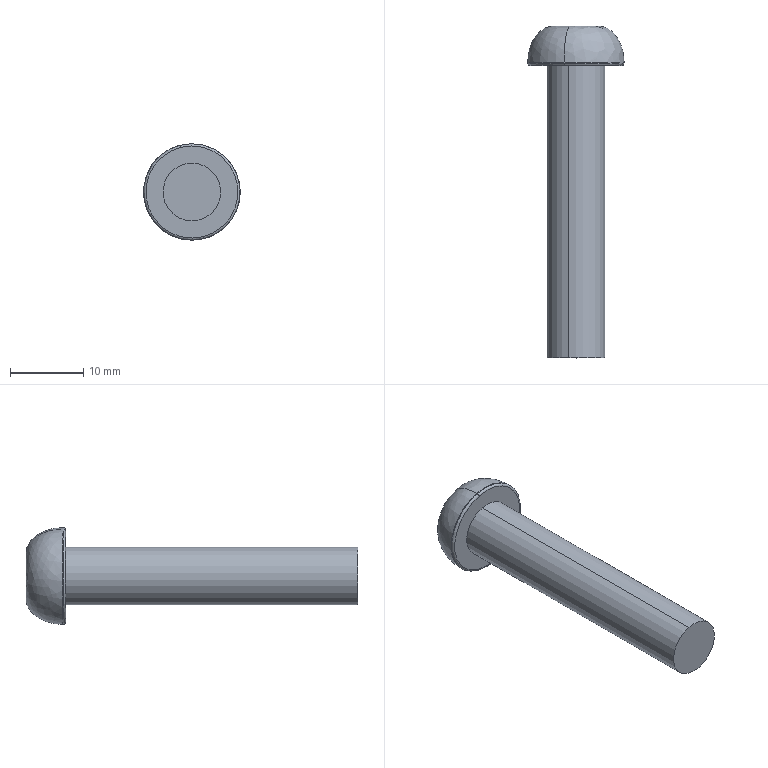Part | SolidWorks | features BaseBody 1 | 1 solid | 23 faces | box 13.2 x 45.4 x 13.2 mm | volume 2505 mm3 | plane 15 | cylinder 4 | torus 2 | spline 2 | commonest cylinder face diameters 7.9 x2 13.2 x2
STEP:
#1=CARTESIAN_POINT('',(-484.292,-107.35,172.017));
#2=VERTEX_POINT('',#1);
#3=CARTESIAN_POINT('',(-486.243,-107.35,179.672));
#4=VERTEX_POINT('',#3);
#5=CARTESIAN_POINT('',(-485.268,-107.35,175.844));
#6=DIRECTION('',(0.,-1.,0.));
#7=DIRECTION('',(0.,0.,-1.));
#8=AXIS2_PLACEMENT_3D('',#5,#6,#7);
#9=CIRCLE('',#8,3.95);
#10=EDGE_CURVE('',#2,#4,#9,.T.);
#11=ORIENTED_EDGE('',*,*,#10,.F.);
#12=CARTESIAN_POINT('',(-484.292,-67.35,172.017));
#13=VERTEX_POINT('',#12);
#14=CARTESIAN_POINT('',(-484.292,-79.35,172.017));
#15=DIRECTION('',(0.,1.,0.));
#16=VECTOR('',#15,1000.);
#17=LINE('',#14,#16);
#18=EDGE_CURVE('',#2,#13,#17,.T.);
#19=ORIENTED_EDGE('',*,*,#18,.T.);
#20=CARTESIAN_POINT('',(-486.243,-67.35,179.672));
#21=VERTEX_POINT('',#20);
#22=CARTESIAN_POINT('',(-485.268,-67.35,175.844));
#23=DIRECTION('',(0.,1.,0.));
#24=DIRECTION('',(0.,0.,-1.));
#25=AXIS2_PLACEMENT_3D('',#22,#23,#24);
#26=CIRCLE('',#25,3.95);
#27=EDGE_CURVE('',#21,#13,#26,.T.);
#28=ORIENTED_EDGE('',*,*,#27,.F.);
#29=CARTESIAN_POINT('',(-486.243,-79.35,179.672));
#30=DIRECTION('',(0.,1.,0.));
#31=VECTOR('',#30,1000.);
#32=LINE('',#29,#31);
#33=EDGE_CURVE('',#4,#21,#32,.T.);
#34=ORIENTED_EDGE('',*,*,#33,.F.);
#35=EDGE_LOOP('',(#11,#19,#28,#34));
#36=FACE_OUTER_BOUND('',#35,.T.);
#37=CARTESIAN_POINT('',(-485.268,-79.35,175.844));
#38=DIRECTION('',(0.,1.,0.));
#39=DIRECTION('',(-0.247,0.,0.969));
#40=AXIS2_PLACEMENT_3D('',#37,#38,#39);
#41=CYLINDRICAL_SURFACE('',#40,3.95);
#42=ADVANCED_FACE('',(#36),#41,.T.);
#43=CARTESIAN_POINT('',(-483.638,-67.05,169.449));
#44=VERTEX_POINT('',#43);
#45=CARTESIAN_POINT('',(-486.898,-67.05,182.24));
#46=VERTEX_POINT('',#45);
#47=CARTESIAN_POINT('',(-485.268,-67.05,175.844));
#48=DIRECTION('',(0.,-1.,0.));
#49=DIRECTION('',(0.247,0.,-0.969));
#50=AXIS2_PLACEMENT_3D('',#47,#48,#49);
#51=CIRCLE('',#50,6.6);
#52=EDGE_CURVE('',#44,#46,#51,.T.);
#53=ORIENTED_EDGE('',*,*,#52,.T.);
#54=CARTESIAN_POINT('',(-486.824,-67.35,181.949));
#55=VERTEX_POINT('',#54);
#56=CARTESIAN_POINT('',(-486.824,-67.05,181.949));
#57=DIRECTION('',(0.969,0.,0.247));
#58=DIRECTION('',(0.247,0.,-0.969));
#59=AXIS2_PLACEMENT_3D('',#56,#57,#58);
#60=CIRCLE('',#59,0.3);
#61=EDGE_CURVE('',#46,#55,#60,.T.);
#62=ORIENTED_EDGE('',*,*,#61,.T.);
#63=CARTESIAN_POINT('',(-483.712,-67.35,169.739));
#64=VERTEX_POINT('',#63);
#65=CARTESIAN_POINT('',(-485.268,-67.35,175.844));
#66=DIRECTION('',(0.,-1.,0.));
#67=DIRECTION('',(0.247,0.,-0.969));
#68=AXIS2_PLACEMENT_3D('',#65,#66,#67);
#69=CIRCLE('',#68,6.3);
#70=EDGE_CURVE('',#64,#55,#69,.T.);
#71=ORIENTED_EDGE('',*,*,#70,.F.);
#72=CARTESIAN_POINT('',(-483.712,-67.05,169.739));
#73=DIRECTION('',(-0.969,0.,-0.247));
#74=DIRECTION('',(-0.247,0.,0.969));
#75=AXIS2_PLACEMENT_3D('',#72,#73,#74);
#76=CIRCLE('',#75,0.3);
#77=EDGE_CURVE('',#44,#64,#76,.T.);
#78=ORIENTED_EDGE('',*,*,#77,.F.);
#79=EDGE_LOOP('',(#53,#62,#71,#78));
#80=FACE_OUTER_BOUND('',#79,.T.);
#81=CARTESIAN_POINT('',(-485.268,-67.05,175.844));
#82=DIRECTION('',(0.,-1.,0.));
#83=DIRECTION('',(0.247,0.,-0.969));
#84=AXIS2_PLACEMENT_3D('',#81,#82,#83);
#85=TOROIDAL_SURFACE('',#84,6.3,0.3);
#86=ADVANCED_FACE('',(#80),#85,.T.);
#87=ORIENTED_EDGE('',*,*,#52,.F.);
#88=CARTESIAN_POINT('',(-483.638,-66.95,169.449));
#89=VERTEX_POINT('',#88);
#90=CARTESIAN_POINT('',(-483.638,-67.35,169.449));
#91=DIRECTION('',(0.,1.,0.));
#92=VECTOR('',#91,1000.);
#93=LINE('',#90,#92);
#94=EDGE_CURVE('',#44,#89,#93,.T.);
#95=ORIENTED_EDGE('',*,*,#94,.T.);
#96=CARTESIAN_POINT('',(-486.898,-66.95,182.24));
#97=VERTEX_POINT('',#96);
#98=CARTESIAN_POINT('',(-486.898,-66.95,182.24));
#99=CARTESIAN_POINT('',(-474.107,-66.95,185.5));
#100=CARTESIAN_POINT('',(-470.847,-66.95,172.709));
#101=CARTESIAN_POINT('',(-483.638,-66.95,169.449));
#102=(BOUNDED_CURVE()B_SPLINE_CURVE(3,(#98,#99,#100,#101),.UNSPECIFIED.,.F.,.F.)B_SPLINE_CURVE_WITH_KNOTS((4,4),(0.,1.),.UNSPECIFIED.)CURVE()GEOMETRIC_REPRESENTATION_ITEM()RATIONAL_B_SPLINE_CURVE((1.,0.3333,0.3333,1.))REPRESENTATION_ITEM(''));
#103=EDGE_CURVE('',#97,#89,#102,.T.);
#104=ORIENTED_EDGE('',*,*,#103,.F.);
#105=CARTESIAN_POINT('',(-486.898,-67.35,182.24));
#106=DIRECTION('',(0.,1.,0.));
#107=VECTOR('',#106,1000.);
#108=LINE('',#105,#107);
#109=EDGE_CURVE('',#46,#97,#108,.T.);
#110=ORIENTED_EDGE('',*,*,#109,.F.);
#111=EDGE_LOOP('',(#87,#95,#104,#110));
#112=FACE_OUTER_BOUND('',#111,.T.);
#113=CARTESIAN_POINT('',(-485.268,-67.35,175.844));
#114=DIRECTION('',(0.,1.,0.));
#115=DIRECTION('',(-0.247,0.,0.969));
#116=AXIS2_PLACEMENT_3D('',#113,#114,#115);
#117=CYLINDRICAL_SURFACE('',#116,6.6);
#118=ADVANCED_FACE('',(#112),#117,.T.);
#119=CARTESIAN_POINT('',(-487.296,-64.03,177.923));
#120=VERTEX_POINT('',#119);
#121=CARTESIAN_POINT('',(-485.268,-65.482,175.844));
#122=VERTEX_POINT('',#121);
#123=CARTESIAN_POINT('',(-487.296,-64.03,177.923));
#124=DIRECTION('',(0.6247,-0.4472,-0.6401));
#125=VECTOR('',#124,1000.);
#126=LINE('',#123,#125);
#127=EDGE_CURVE('',#120,#122,#126,.T.);
#128=ORIENTED_EDGE('',*,*,#127,.T.);
#129=CARTESIAN_POINT('',(-488.082,-64.03,175.127));
#130=VERTEX_POINT('',#129);
#131=CARTESIAN_POINT('',(-488.082,-64.03,175.127));
#132=DIRECTION('',(0.8667,-0.4472,0.2209));
#133=VECTOR('',#132,1000.);
#134=LINE('',#131,#133);
#135=EDGE_CURVE('',#130,#122,#134,.T.);
#136=ORIENTED_EDGE('',*,*,#135,.F.);
#137=CARTESIAN_POINT('',(-488.082,-64.03,175.127));
#138=DIRECTION('',(0.2706,0.,0.9627));
#139=VECTOR('',#138,1000.);
#140=LINE('',#137,#139);
#141=EDGE_CURVE('',#130,#120,#140,.T.);
#142=ORIENTED_EDGE('',*,*,#141,.T.);
#143=EDGE_LOOP('',(#128,#136,#142));
#144=FACE_OUTER_BOUND('',#143,.T.);
#145=CARTESIAN_POINT('',(-488.082,-64.03,175.127));
#146=DIRECTION('',(-0.4813,-0.866,0.1353));
#147=DIRECTION('',(-0.8741,0.4858,0.));
#148=AXIS2_PLACEMENT_3D('',#145,#146,#147);
#149=PLANE('',#148);
#150=ADVANCED_FACE('',(#144),#149,.F.);
#151=CARTESIAN_POINT('',(-487.296,-61.95,177.923));
#152=VERTEX_POINT('',#151);
#153=CARTESIAN_POINT('',(-487.296,-61.95,177.923));
#154=DIRECTION('',(0.,-1.,0.));
#155=VECTOR('',#154,1000.);
#156=LINE('',#153,#155);
#157=EDGE_CURVE('',#152,#120,#156,.T.);
#158=ORIENTED_EDGE('',*,*,#157,.T.);
#159=ORIENTED_EDGE('',*,*,#141,.F.);
#160=CARTESIAN_POINT('',(-488.082,-61.95,175.127));
#161=VERTEX_POINT('',#160);
#162=CARTESIAN_POINT('',(-488.082,-61.95,175.127));
#163=DIRECTION('',(0.,-1.,0.));
#164=VECTOR('',#163,1000.);
#165=LINE('',#162,#164);
#166=EDGE_CURVE('',#161,#130,#165,.T.);
#167=ORIENTED_EDGE('',*,*,#166,.F.);
#168=CARTESIAN_POINT('',(-487.296,-61.95,177.923));
#169=DIRECTION('',(-0.2706,0.,-0.9627));
#170=VECTOR('',#169,1000.);
#171=LINE('',#168,#170);
#172=EDGE_CURVE('',#152,#161,#171,.T.);
#173=ORIENTED_EDGE('',*,*,#172,.F.);
#174=EDGE_LOOP('',(#158,#159,#167,#173));
#175=FACE_OUTER_BOUND('',#174,.T.);
#176=CARTESIAN_POINT('',(-488.082,-64.03,175.127));
#177=DIRECTION('',(-0.9627,0.,0.2706));
#178=DIRECTION('',(0.,1.,0.));
#179=AXIS2_PLACEMENT_3D('',#176,#177,#178);
#180=PLANE('',#179);
#181=ADVANCED_FACE('',(#175),#180,.F.);
#182=CARTESIAN_POINT('',(-482.454,-61.95,176.562));
#183=VERTEX_POINT('',#182);
#184=CARTESIAN_POINT('',(-484.482,-61.95,178.64));
#185=VERTEX_POINT('',#184);
#186=CARTESIAN_POINT('',(-482.454,-61.95,176.562));
#187=DIRECTION('',(-0.6984,0.,0.7157));
#188=VECTOR('',#187,1000.);
#189=LINE('',#186,#188);
#190=EDGE_CURVE('',#183,#185,#189,.T.);
#191=ORIENTED_EDGE('',*,*,#190,.T.);
#192=CARTESIAN_POINT('',(-484.482,-61.95,178.64));
#193=DIRECTION('',(-0.969,0.,-0.247));
#194=VECTOR('',#193,1000.);
#195=LINE('',#192,#194);
#196=EDGE_CURVE('',#185,#152,#195,.T.);
#197=ORIENTED_EDGE('',*,*,#196,.T.);
#198=ORIENTED_EDGE('',*,*,#172,.T.);
#199=CARTESIAN_POINT('',(-486.054,-61.95,173.049));
#200=VERTEX_POINT('',#199);
#201=CARTESIAN_POINT('',(-488.082,-61.95,175.127));
#202=DIRECTION('',(0.6984,0.,-0.7157));
#203=VECTOR('',#202,1000.);
#204=LINE('',#201,#203);
#205=EDGE_CURVE('',#161,#200,#204,.T.);
#206=ORIENTED_EDGE('',*,*,#205,.T.);
#207=CARTESIAN_POINT('',(-483.239,-61.95,173.766));
#208=VERTEX_POINT('',#207);
#209=CARTESIAN_POINT('',(-486.054,-61.95,173.049));
#210=DIRECTION('',(0.969,0.,0.247));
#211=VECTOR('',#210,1000.);
#212=LINE('',#209,#211);
#213=EDGE_CURVE('',#200,#208,#212,.T.);
#214=ORIENTED_EDGE('',*,*,#213,.T.);
#215=CARTESIAN_POINT('',(-483.239,-61.95,173.766));
#216=DIRECTION('',(0.2706,0.,0.9627));
#217=VECTOR('',#216,1000.);
#218=LINE('',#215,#217);
#219=EDGE_CURVE('',#208,#183,#218,.T.);
#220=ORIENTED_EDGE('',*,*,#219,.T.);
#221=EDGE_LOOP('',(#191,#197,#198,#206,#214,#220));
#222=FACE_BOUND('',#221,.T.);
#223=CARTESIAN_POINT('',(-484.502,-61.95,172.84));
#224=VERTEX_POINT('',#223);
#225=CARTESIAN_POINT('',(-486.033,-61.95,178.848));
#226=VERTEX_POINT('',#225);
#227=CARTESIAN_POINT('',(-484.502,-61.95,172.84));
#228=CARTESIAN_POINT('',(-484.6,-61.95,172.815));
#229=CARTESIAN_POINT('',(-484.699,-61.95,172.795));
#230=CARTESIAN_POINT('',(-484.899,-61.95,172.765));
#231=CARTESIAN_POINT('',(-485.002,-61.95,172.755));
#232=CARTESIAN_POINT('',(-485.305,-61.95,172.74));
#233=CARTESIAN_POINT('',(-485.509,-61.95,172.75));
#234=CARTESIAN_POINT('',(-485.911,-61.95,172.808));
#235=CARTESIAN_POINT('',(-486.107,-61.95,172.855));
#236=CARTESIAN_POINT('',(-486.492,-61.95,172.99));
#237=CARTESIAN_POINT('',(-486.677,-61.95,173.076));
#238=CARTESIAN_POINT('',(-486.937,-61.95,173.23));
#239=CARTESIAN_POINT('',(-487.021,-61.95,173.286));
#240=CARTESIAN_POINT('',(-487.184,-61.95,173.406));
#241=CARTESIAN_POINT('',(-487.264,-61.95,173.472));
#242=CARTESIAN_POINT('',(-487.489,-61.95,173.675));
#243=CARTESIAN_POINT('',(-487.626,-61.95,173.826));
#244=CARTESIAN_POINT('',(-487.87,-61.95,174.152));
#245=CARTESIAN_POINT('',(-487.974,-61.95,174.324));
#246=CARTESIAN_POINT('',(-488.152,-61.95,174.692));
#247=CARTESIAN_POINT('',(-488.222,-61.95,174.884));
#248=CARTESIAN_POINT('',(-488.297,-61.95,175.176));
#249=CARTESIAN_POINT('',(-488.317,-61.95,175.275));
#250=CARTESIAN_POINT('',(-488.347,-61.95,175.475));
#251=CARTESIAN_POINT('',(-488.357,-61.95,175.579));
#252=CARTESIAN_POINT('',(-488.372,-61.95,175.881));
#253=CARTESIAN_POINT('',(-488.362,-61.95,176.085));
#254=CARTESIAN_POINT('',(-488.304,-61.95,176.487));
#255=CARTESIAN_POINT('',(-488.257,-61.95,176.683));
#256=CARTESIAN_POINT('',(-488.122,-61.95,177.069));
#257=CARTESIAN_POINT('',(-488.036,-61.95,177.254));
#258=CARTESIAN_POINT('',(-487.882,-61.95,177.514));
#259=CARTESIAN_POINT('',(-487.826,-61.95,177.598));
#260=CARTESIAN_POINT('',(-487.706,-61.95,177.76));
#261=CARTESIAN_POINT('',(-487.64,-61.95,177.841));
#262=CARTESIAN_POINT('',(-487.437,-61.95,178.065));
#263=CARTESIAN_POINT('',(-487.287,-61.95,178.202));
#264=CARTESIAN_POINT('',(-486.961,-61.95,178.446));
#265=CARTESIAN_POINT('',(-486.79,-61.95,178.551));
#266=CARTESIAN_POINT('',(-486.421,-61.95,178.729));
#267=CARTESIAN_POINT('',(-486.23,-61.95,178.798));
#268=CARTESIAN_POINT('',(-486.033,-61.95,178.848));
#269=B_SPLINE_CURVE_WITH_KNOTS('',3,(#227,#228,#229,#230,#231,#232,#233,#234,#235,#236,#237,#238,#239,#240,#241,#242,#243,#244,#245,#246,#247,#248,#249,#250,#251,#252,#253,#254,#255,#256,#257,#258,#259,#260,#261,#262,#263,#264,#265,#266,#267,#268),.UNSPECIFIED.,.F.,.F.,(4,2,2,2,2,2,2,2,2,2,2,2,2,2,2,2,2,2,2,2,4),(0.,0.03125,0.0625,0.125,0.1875,0.25,0.2813,0.3125,0.375,0.4375,0.5,0.5313,0.5625,0.625,0.6875,0.75,0.7813,0.8125,0.875,0.9375,1.),.UNSPECIFIED.);
#270=EDGE_CURVE('',#224,#226,#269,.T.);
#271=ORIENTED_EDGE('',*,*,#270,.T.);
#272=CARTESIAN_POINT('',(-486.033,-61.95,178.848));
#273=CARTESIAN_POINT('',(-485.935,-61.95,178.873));
#274=CARTESIAN_POINT('',(-485.836,-61.95,178.893));
#275=CARTESIAN_POINT('',(-485.636,-61.95,178.923));
#276=CARTESIAN_POINT('',(-485.533,-61.95,178.933));
#277=CARTESIAN_POINT('',(-485.23,-61.95,178.949));
#278=CARTESIAN_POINT('',(-485.027,-61.95,178.939));
#279=CARTESIAN_POINT('',(-484.625,-61.95,178.881));
#280=CARTESIAN_POINT('',(-484.429,-61.95,178.833));
#281=CARTESIAN_POINT('',(-484.043,-61.95,178.699));
#282=CARTESIAN_POINT('',(-483.858,-61.95,178.612));
#283=CARTESIAN_POINT('',(-483.598,-61.95,178.458));
#284=CARTESIAN_POINT('',(-483.514,-61.95,178.403));
#285=CARTESIAN_POINT('',(-483.352,-61.95,178.282));
#286=CARTESIAN_POINT('',(-483.271,-61.95,178.216));
#287=CARTESIAN_POINT('',(-483.047,-61.95,178.013));
#288=CARTESIAN_POINT('',(-482.909,-61.95,177.862));
#289=CARTESIAN_POINT('',(-482.666,-61.95,177.537));
#290=CARTESIAN_POINT('',(-482.561,-61.95,177.365));
#291=CARTESIAN_POINT('',(-482.383,-61.95,176.997));
#292=CARTESIAN_POINT('',(-482.314,-61.95,176.805));
#293=CARTESIAN_POINT('',(-482.239,-61.95,176.512));
#294=CARTESIAN_POINT('',(-482.219,-61.95,176.414));
#295=CARTESIAN_POINT('',(-482.189,-61.95,176.213));
#296=CARTESIAN_POINT('',(-482.179,-61.95,176.11));
#297=CARTESIAN_POINT('',(-482.163,-61.95,175.807));
#298=CARTESIAN_POINT('',(-482.173,-61.95,175.604));
#299=CARTESIAN_POINT('',(-482.231,-61.95,175.201));
#300=CARTESIAN_POINT('',(-482.279,-61.95,175.006));
#301=CARTESIAN_POINT('',(-482.413,-61.95,174.62));
#302=CARTESIAN_POINT('',(-482.499,-61.95,174.435));
#303=CARTESIAN_POINT('',(-482.654,-61.95,174.175));
#304=CARTESIAN_POINT('',(-482.709,-61.95,174.091));
#305=CARTESIAN_POINT('',(-482.83,-61.95,173.928));
#306=CARTESIAN_POINT('',(-482.895,-61.95,173.848));
#307=CARTESIAN_POINT('',(-483.098,-61.95,173.623));
#308=CARTESIAN_POINT('',(-483.249,-61.95,173.486));
#309=CARTESIAN_POINT('',(-483.574,-61.95,173.243));
#310=CARTESIAN_POINT('',(-483.746,-61.95,173.138));
#311=CARTESIAN_POINT('',(-484.115,-61.95,172.96));
#312=CARTESIAN_POINT('',(-484.305,-61.95,172.89));
#313=CARTESIAN_POINT('',(-484.502,-61.95,172.84));
#314=B_SPLINE_CURVE_WITH_KNOTS('',3,(#272,#273,#274,#275,#276,#277,#278,#279,#280,#281,#282,#283,#284,#285,#286,#287,#288,#289,#290,#291,#292,#293,#294,#295,#296,#297,#298,#299,#300,#301,#302,#303,#304,#305,#306,#307,#308,#309,#310,#311,#312,#313),.UNSPECIFIED.,.F.,.F.,(4,2,2,2,2,2,2,2,2,2,2,2,2,2,2,2,2,2,2,2,4),(0.,0.03125,0.0625,0.125,0.1875,0.25,0.2812,0.3125,0.375,0.4375,0.5,0.5312,0.5625,0.625,0.6875,0.75,0.7812,0.8125,0.875,0.9375,1.),.UNSPECIFIED.);
#315=EDGE_CURVE('',#226,#224,#314,.T.);
#316=ORIENTED_EDGE('',*,*,#315,.T.);
#317=EDGE_LOOP('',(#271,#316));
#318=FACE_OUTER_BOUND('',#317,.T.);
#319=CARTESIAN_POINT('',(-485.268,-61.95,175.844));
#320=DIRECTION('',(0.,-1.,0.));
#321=DIRECTION('',(0.,0.,-1.));
#322=AXIS2_PLACEMENT_3D('',#319,#320,#321);
#323=PLANE('',#322);
#324=ADVANCED_FACE('',(#222,#318),#323,.F.);
#325=CARTESIAN_POINT('',(-483.638,-66.95,169.449));
#326=CARTESIAN_POINT('',(-483.638,-66.369,169.449));
#327=CARTESIAN_POINT('',(-483.665,-65.419,169.557));
#328=CARTESIAN_POINT('',(-483.772,-64.203,169.977));
#329=CARTESIAN_POINT('',(-483.888,-63.376,170.432));
#330=CARTESIAN_POINT('',(-484.032,-62.71,170.996));
#331=CARTESIAN_POINT('',(-484.241,-62.104,171.816));
#332=CARTESIAN_POINT('',(-484.403,-61.95,172.453));
#333=CARTESIAN_POINT('',(-484.502,-61.95,172.84));
#334=(BOUNDED_CURVE()B_SPLINE_CURVE(3,(#325,#326,#327,#328,#329,#330,#331,#332,#333),.UNSPECIFIED.,.F.,.F.)B_SPLINE_CURVE_WITH_KNOTS((4,1,1,1,1,1,4),(0.,0.2462,0.3741,0.502,0.6299,0.7578,1.),.UNSPECIFIED.)CURVE()GEOMETRIC_REPRESENTATION_ITEM()RATIONAL_B_SPLINE_CURVE((1.,1.,1.,1.,1.,1.,1.,1.,1.))REPRESENTATION_ITEM(''));
#335=EDGE_CURVE('',#89,#224,#334,.T.);
#336=ORIENTED_EDGE('',*,*,#335,.T.);
#337=ORIENTED_EDGE('',*,*,#315,.F.);
#338=CARTESIAN_POINT('',(-486.898,-66.95,182.24));
#339=CARTESIAN_POINT('',(-486.898,-66.369,182.239));
#340=CARTESIAN_POINT('',(-486.87,-65.419,182.132));
#341=CARTESIAN_POINT('',(-486.763,-64.203,181.712));
#342=CARTESIAN_POINT('',(-486.647,-63.376,181.256));
#343=CARTESIAN_POINT('',(-486.503,-62.71,180.692));
#344=CARTESIAN_POINT('',(-486.295,-62.104,179.873));
#345=CARTESIAN_POINT('',(-486.132,-61.95,179.236));
#346=CARTESIAN_POINT('',(-486.033,-61.95,178.848));
#347=B_SPLINE_CURVE_WITH_KNOTS('',3,(#338,#339,#340,#341,#342,#343,#344,#345,#346),.UNSPECIFIED.,.F.,.F.,(4,1,1,1,1,1,4),(0.,0.2462,0.3741,0.502,0.6299,0.7578,1.),.UNSPECIFIED.);
#348=EDGE_CURVE('',#97,#226,#347,.T.);
#349=ORIENTED_EDGE('',*,*,#348,.F.);
#350=ORIENTED_EDGE('',*,*,#103,.T.);
#351=EDGE_LOOP('',(#336,#337,#349,#350));
#352=FACE_OUTER_BOUND('',#351,.T.);
#353=CARTESIAN_POINT('',(-486.898,-66.95,182.24));
#354=CARTESIAN_POINT('',(-474.107,-66.95,185.5));
#355=CARTESIAN_POINT('',(-470.847,-66.95,172.709));
#356=CARTESIAN_POINT('',(-483.638,-66.95,169.449));
#357=CARTESIAN_POINT('',(-486.898,-66.369,182.239));
#358=CARTESIAN_POINT('',(-474.107,-66.369,185.5));
#359=CARTESIAN_POINT('',(-470.847,-66.369,172.709));
#360=CARTESIAN_POINT('',(-483.638,-66.369,169.449));
#361=CARTESIAN_POINT('',(-486.87,-65.419,182.132));
#362=CARTESIAN_POINT('',(-474.295,-65.419,185.337));
#363=CARTESIAN_POINT('',(-471.09,-65.419,172.762));
#364=CARTESIAN_POINT('',(-483.665,-65.419,169.557));
#365=CARTESIAN_POINT('',(-486.763,-64.203,181.712));
#366=CARTESIAN_POINT('',(-475.028,-64.203,184.703));
#367=CARTESIAN_POINT('',(-472.037,-64.203,172.968));
#368=CARTESIAN_POINT('',(-483.772,-64.203,169.977));
#369=CARTESIAN_POINT('',(-486.647,-63.376,181.256));
#370=CARTESIAN_POINT('',(-475.823,-63.376,184.015));
#371=CARTESIAN_POINT('',(-473.064,-63.376,173.191));
#372=CARTESIAN_POINT('',(-483.888,-63.376,170.432));
#373=CARTESIAN_POINT('',(-486.503,-62.71,180.692));
#374=CARTESIAN_POINT('',(-476.807,-62.71,183.164));
#375=CARTESIAN_POINT('',(-474.335,-62.71,173.468));
#376=CARTESIAN_POINT('',(-484.032,-62.71,170.996));
#377=CARTESIAN_POINT('',(-486.292,-62.096,179.862));
#378=CARTESIAN_POINT('',(-478.257,-62.096,181.91));
#379=CARTESIAN_POINT('',(-476.209,-62.096,173.875));
#380=CARTESIAN_POINT('',(-484.244,-62.096,171.827));
#381=CARTESIAN_POINT('',(-486.126,-61.945,179.213));
#382=CARTESIAN_POINT('',(-479.389,-61.945,180.931));
#383=CARTESIAN_POINT('',(-477.671,-61.945,174.193));
#384=CARTESIAN_POINT('',(-484.409,-61.945,172.475));
#385=CARTESIAN_POINT('',(-486.025,-61.95,178.817));
#386=CARTESIAN_POINT('',(-480.08,-61.95,180.332));
#387=CARTESIAN_POINT('',(-478.565,-61.95,174.387));
#388=CARTESIAN_POINT('',(-484.51,-61.95,172.872));
#389=(BOUNDED_SURFACE()B_SPLINE_SURFACE(3,3,((#353,#354,#355,#356),(#357,#358,#359,#360),(#361,#362,#363,#364),(#365,#366,#367,#368),(#369,#370,#371,#372),(#373,#374,#375,#376),(#377,#378,#379,#380),(#381,#382,#383,#384),(#385,#386,#387,#388)),.UNSPECIFIED.,.F.,.F.,.F.)B_SPLINE_SURFACE_WITH_KNOTS((4,1,1,1,1,1,4),(4,4),(0.009324,0.25,0.375,0.5,0.625,0.75,0.9931),(0.,1.),.UNSPECIFIED.)GEOMETRIC_REPRESENTATION_ITEM()RATIONAL_B_SPLINE_SURFACE(((1.,0.3333,0.3333,1.),(1.,0.3333,0.3333,1.),(1.,0.3333,0.3333,1.),(1.,0.3333,0.3333,1.),(1.,0.3333,0.3333,1.),(1.,0.3333,0.3333,1.),(1.,0.3333,0.3333,1.),(1.,0.3333,0.3333,1.),(1.,0.3333,0.3333,1.)))REPRESENTATION_ITEM('')SURFACE());
#390=ADVANCED_FACE('',(#352),#389,.F.);
#391=ORIENTED_EDGE('',*,*,#94,.F.);
#392=CARTESIAN_POINT('',(-485.268,-67.05,175.844));
#393=DIRECTION('',(0.,-1.,0.));
#394=DIRECTION('',(0.247,0.,-0.969));
#395=AXIS2_PLACEMENT_3D('',#392,#393,#394);
#396=CIRCLE('',#395,6.6);
#397=EDGE_CURVE('',#46,#44,#396,.T.);
#398=ORIENTED_EDGE('',*,*,#397,.F.);
#399=ORIENTED_EDGE('',*,*,#109,.T.);
#400=CARTESIAN_POINT('',(-483.638,-66.95,169.449));
#401=CARTESIAN_POINT('',(-487.384,-66.95,168.494));
#402=CARTESIAN_POINT('',(-490.708,-66.95,170.468));
#403=CARTESIAN_POINT('',(-491.663,-66.95,174.214));
#404=CARTESIAN_POINT('',(-492.618,-66.95,177.96));
#405=CARTESIAN_POINT('',(-490.644,-66.95,181.285));
#406=CARTESIAN_POINT('',(-486.898,-66.95,182.24));
#407=(BOUNDED_CURVE()B_SPLINE_CURVE(3,(#400,#401,#402,#403,#404,#405,#406),.UNSPECIFIED.,.F.,.T.)B_SPLINE_CURVE_WITH_KNOTS((4,3,4),(0.,0.5,1.),.UNSPECIFIED.)CURVE()GEOMETRIC_REPRESENTATION_ITEM()RATIONAL_B_SPLINE_CURVE((1.,0.8047,0.8047,1.,0.8047,0.8047,1.))REPRESENTATION_ITEM(''));
#408=EDGE_CURVE('',#89,#97,#407,.T.);
#409=ORIENTED_EDGE('',*,*,#408,.F.);
#410=EDGE_LOOP('',(#391,#398,#399,#409));
#411=FACE_OUTER_BOUND('',#410,.T.);
#412=CARTESIAN_POINT('',(-485.268,-67.35,175.844));
#413=DIRECTION('',(0.,1.,0.));
#414=DIRECTION('',(-0.247,0.,0.969));
#415=AXIS2_PLACEMENT_3D('',#412,#413,#414);
#416=CYLINDRICAL_SURFACE('',#415,6.6);
#417=ADVANCED_FACE('',(#411),#416,.T.);
#418=ORIENTED_EDGE('',*,*,#61,.F.);
#419=ORIENTED_EDGE('',*,*,#397,.T.);
#420=ORIENTED_EDGE('',*,*,#77,.T.);
#421=CARTESIAN_POINT('',(-485.268,-67.35,175.844));
#422=DIRECTION('',(0.,-1.,0.));
#423=DIRECTION('',(0.247,0.,-0.969));
#424=AXIS2_PLACEMENT_3D('',#421,#422,#423);
#425=CIRCLE('',#424,6.3);
#426=EDGE_CURVE('',#55,#64,#425,.T.);
#427=ORIENTED_EDGE('',*,*,#426,.F.);
#428=EDGE_LOOP('',(#418,#419,#420,#427));
#429=FACE_OUTER_BOUND('',#428,.T.);
#430=CARTESIAN_POINT('',(-485.268,-67.05,175.844));
#431=DIRECTION('',(0.,-1.,0.));
#432=DIRECTION('',(0.247,0.,-0.969));
#433=AXIS2_PLACEMENT_3D('',#430,#431,#432);
#434=TOROIDAL_SURFACE('',#433,6.3,0.3);
#435=ADVANCED_FACE('',(#429),#434,.T.);
#436=ORIENTED_EDGE('',*,*,#27,.T.);
#437=CARTESIAN_POINT('',(-485.268,-67.35,175.844));
#438=DIRECTION('',(0.,1.,0.));
#439=DIRECTION('',(0.,0.,-1.));
#440=AXIS2_PLACEMENT_3D('',#437,#438,#439);
#441=CIRCLE('',#440,3.95);
#442=EDGE_CURVE('',#13,#21,#441,.T.);
#443=ORIENTED_EDGE('',*,*,#442,.T.);
#444=EDGE_LOOP('',(#436,#443));
#445=FACE_BOUND('',#444,.T.);
#446=ORIENTED_EDGE('',*,*,#70,.T.);
#447=ORIENTED_EDGE('',*,*,#426,.T.);
#448=EDGE_LOOP('',(#446,#447));
#449=FACE_OUTER_BOUND('',#448,.T.);
#450=CARTESIAN_POINT('',(-485.268,-67.35,175.844));
#451=DIRECTION('',(0.,-1.,0.));
#452=DIRECTION('',(0.,0.,-1.));
#453=AXIS2_PLACEMENT_3D('',#450,#451,#452);
#454=PLANE('',#453);
#455=ADVANCED_FACE('',(#445,#449),#454,.T.);
#456=ORIENTED_EDGE('',*,*,#18,.F.);
#457=CARTESIAN_POINT('',(-485.268,-107.35,175.844));
#458=DIRECTION('',(0.,-1.,0.));
#459=DIRECTION('',(0.,0.,-1.));
#460=AXIS2_PLACEMENT_3D('',#457,#458,#459);
#461=CIRCLE('',#460,3.95);
#462=EDGE_CURVE('',#4,#2,#461,.T.);
#463=ORIENTED_EDGE('',*,*,#462,.F.);
#464=ORIENTED_EDGE('',*,*,#33,.T.);
#465=ORIENTED_EDGE('',*,*,#442,.F.);
#466=EDGE_LOOP('',(#456,#463,#464,#465));
#467=FACE_OUTER_BOUND('',#466,.T.);
#468=CARTESIAN_POINT('',(-485.268,-79.35,175.844));
#469=DIRECTION('',(0.,1.,0.));
#470=DIRECTION('',(-0.247,0.,0.969));
#471=AXIS2_PLACEMENT_3D('',#468,#469,#470);
#472=CYLINDRICAL_SURFACE('',#471,3.95);
#473=ADVANCED_FACE('',(#467),#472,.T.);
#474=ORIENTED_EDGE('',*,*,#408,.T.);
#475=ORIENTED_EDGE('',*,*,#348,.T.);
#476=ORIENTED_EDGE('',*,*,#270,.F.);
#477=ORIENTED_EDGE('',*,*,#335,.F.);
#478=EDGE_LOOP('',(#474,#475,#476,#477));
#479=FACE_OUTER_BOUND('',#478,.T.);
#480=CARTESIAN_POINT('',(-483.638,-66.95,169.449));
#481=CARTESIAN_POINT('',(-487.384,-66.95,168.494));
#482=CARTESIAN_POINT('',(-490.708,-66.95,170.468));
#483=CARTESIAN_POINT('',(-491.663,-66.95,174.214));
#484=CARTESIAN_POINT('',(-492.618,-66.95,177.96));
#485=CARTESIAN_POINT('',(-490.644,-66.95,181.285));
#486=CARTESIAN_POINT('',(-486.898,-66.95,182.24));
#487=CARTESIAN_POINT('',(-483.638,-66.369,169.449));
#488=CARTESIAN_POINT('',(-487.384,-66.369,168.494));
#489=CARTESIAN_POINT('',(-490.708,-66.369,170.468));
#490=CARTESIAN_POINT('',(-491.663,-66.369,174.214));
#491=CARTESIAN_POINT('',(-492.618,-66.369,177.96));
#492=CARTESIAN_POINT('',(-490.644,-66.369,181.285));
#493=CARTESIAN_POINT('',(-486.898,-66.369,182.239));
#494=CARTESIAN_POINT('',(-483.665,-65.419,169.557));
#495=CARTESIAN_POINT('',(-487.348,-65.419,168.618));
#496=CARTESIAN_POINT('',(-490.617,-65.419,170.558));
#497=CARTESIAN_POINT('',(-491.555,-65.419,174.242));
#498=CARTESIAN_POINT('',(-492.494,-65.419,177.925));
#499=CARTESIAN_POINT('',(-490.554,-65.419,181.193));
#500=CARTESIAN_POINT('',(-486.87,-65.419,182.132));
#501=CARTESIAN_POINT('',(-483.772,-64.203,169.977));
#502=CARTESIAN_POINT('',(-487.209,-64.203,169.101));
#503=CARTESIAN_POINT('',(-490.259,-64.203,170.911));
#504=CARTESIAN_POINT('',(-491.135,-64.203,174.349));
#505=CARTESIAN_POINT('',(-492.011,-64.203,177.786));
#506=CARTESIAN_POINT('',(-490.201,-64.203,180.836));
#507=CARTESIAN_POINT('',(-486.763,-64.203,181.712));
#508=CARTESIAN_POINT('',(-483.888,-63.376,170.432));
#509=CARTESIAN_POINT('',(-487.059,-63.376,169.624));
#510=CARTESIAN_POINT('',(-489.872,-63.376,171.294));
#511=CARTESIAN_POINT('',(-490.68,-63.376,174.465));
#512=CARTESIAN_POINT('',(-491.488,-63.376,177.635));
#513=CARTESIAN_POINT('',(-489.818,-63.376,180.448));
#514=CARTESIAN_POINT('',(-486.647,-63.376,181.256));
#515=CARTESIAN_POINT('',(-484.032,-62.71,170.996));
#516=CARTESIAN_POINT('',(-486.872,-62.71,170.272));
#517=CARTESIAN_POINT('',(-489.392,-62.71,171.768));
#518=CARTESIAN_POINT('',(-490.116,-62.71,174.608));
#519=CARTESIAN_POINT('',(-490.84,-62.71,177.449));
#520=CARTESIAN_POINT('',(-489.344,-62.71,179.969));
#521=CARTESIAN_POINT('',(-486.503,-62.71,180.692));
#522=CARTESIAN_POINT('',(-484.244,-62.096,171.827));
#523=CARTESIAN_POINT('',(-486.597,-62.096,171.227));
#524=CARTESIAN_POINT('',(-488.685,-62.096,172.467));
#525=CARTESIAN_POINT('',(-489.285,-62.096,174.82));
#526=CARTESIAN_POINT('',(-489.885,-62.096,177.174));
#527=CARTESIAN_POINT('',(-488.645,-62.096,179.262));
#528=CARTESIAN_POINT('',(-486.292,-62.096,179.862));
#529=CARTESIAN_POINT('',(-484.409,-61.945,172.475));
#530=CARTESIAN_POINT('',(-486.382,-61.945,171.972));
#531=CARTESIAN_POINT('',(-488.134,-61.945,173.012));
#532=CARTESIAN_POINT('',(-488.637,-61.945,174.986));
#533=CARTESIAN_POINT('',(-489.14,-61.945,176.959));
#534=CARTESIAN_POINT('',(-488.1,-61.945,178.71));
#535=CARTESIAN_POINT('',(-486.126,-61.945,179.213));
#536=CARTESIAN_POINT('',(-484.51,-61.95,172.872));
#537=CARTESIAN_POINT('',(-486.251,-61.95,172.428));
#538=CARTESIAN_POINT('',(-487.796,-61.95,173.345));
#539=CARTESIAN_POINT('',(-488.24,-61.95,175.087));
#540=CARTESIAN_POINT('',(-488.684,-61.95,176.828));
#541=CARTESIAN_POINT('',(-487.767,-61.95,178.373));
#542=CARTESIAN_POINT('',(-486.025,-61.95,178.817));
#543=(BOUNDED_SURFACE()B_SPLINE_SURFACE(3,3,((#480,#481,#482,#483,#484,#485,#486),(#487,#488,#489,#490,#491,#492,#493),(#494,#495,#496,#497,#498,#499,#500),(#501,#502,#503,#504,#505,#506,#507),(#508,#509,#510,#511,#512,#513,#514),(#515,#516,#517,#518,#519,#520,#521),(#522,#523,#524,#525,#526,#527,#528),(#529,#530,#531,#532,#533,#534,#535),(#536,#537,#538,#539,#540,#541,#542)),.UNSPECIFIED.,.F.,.F.,.F.)B_SPLINE_SURFACE_WITH_KNOTS((4,1,1,1,1,1,4),(4,3,4),(0.009324,0.25,0.375,0.5,0.625,0.75,0.9931),(0.,0.5,1.),.UNSPECIFIED.)GEOMETRIC_REPRESENTATION_ITEM()RATIONAL_B_SPLINE_SURFACE(((1.,0.8047,0.8047,1.,0.8047,0.8047,1.),(1.,0.8047,0.8047,1.,0.8047,0.8047,1.),(1.,0.8047,0.8047,1.,0.8047,0.8047,1.),(1.,0.8047,0.8047,1.,0.8047,0.8047,1.),(1.,0.8047,0.8047,1.,0.8047,0.8047,1.),(1.,0.8047,0.8047,1.,0.8047,0.8047,1.),(1.,0.8047,0.8047,1.,0.8047,0.8047,1.),(1.,0.8047,0.8047,1.,0.8047,0.8047,1.),(1.,0.8047,0.8047,1.,0.8047,0.8047,1.)))REPRESENTATION_ITEM('')SURFACE());
#544=ADVANCED_FACE('',(#479),#543,.F.);
#545=CARTESIAN_POINT('',(-483.239,-64.03,173.766));
#546=VERTEX_POINT('',#545);
#547=CARTESIAN_POINT('',(-483.239,-61.95,173.766));
#548=DIRECTION('',(0.,-1.,0.));
#549=VECTOR('',#548,1000.);
#550=LINE('',#547,#549);
#551=EDGE_CURVE('',#208,#546,#550,.T.);
#552=ORIENTED_EDGE('',*,*,#551,.T.);
#553=CARTESIAN_POINT('',(-482.454,-64.03,176.562));
#554=VERTEX_POINT('',#553);
#555=CARTESIAN_POINT('',(-482.454,-64.03,176.562));
#556=DIRECTION('',(-0.2706,0.,-0.9627));
#557=VECTOR('',#556,1000.);
#558=LINE('',#555,#557);
#559=EDGE_CURVE('',#554,#546,#558,.T.);
#560=ORIENTED_EDGE('',*,*,#559,.F.);
#561=CARTESIAN_POINT('',(-482.454,-61.95,176.562));
#562=DIRECTION('',(0.,-1.,0.));
#563=VECTOR('',#562,1000.);
#564=LINE('',#561,#563);
#565=EDGE_CURVE('',#183,#554,#564,.T.);
#566=ORIENTED_EDGE('',*,*,#565,.F.);
#567=ORIENTED_EDGE('',*,*,#219,.F.);
#568=EDGE_LOOP('',(#552,#560,#566,#567));
#569=FACE_OUTER_BOUND('',#568,.T.);
#570=CARTESIAN_POINT('',(-482.454,-64.03,176.562));
#571=DIRECTION('',(0.9627,0.,-0.2706));
#572=DIRECTION('',(0.,-1.,0.));
#573=AXIS2_PLACEMENT_3D('',#570,#571,#572);
#574=PLANE('',#573);
#575=ADVANCED_FACE('',(#569),#574,.F.);
#576=ORIENTED_EDGE('',*,*,#565,.T.);
#577=CARTESIAN_POINT('',(-484.482,-64.03,178.64));
#578=VERTEX_POINT('',#577);
#579=CARTESIAN_POINT('',(-484.482,-64.03,178.64));
#580=DIRECTION('',(0.6984,0.,-0.7157));
#581=VECTOR('',#580,1000.);
#582=LINE('',#579,#581);
#583=EDGE_CURVE('',#578,#554,#582,.T.);
#584=ORIENTED_EDGE('',*,*,#583,.F.);
#585=CARTESIAN_POINT('',(-484.482,-61.95,178.64));
#586=DIRECTION('',(0.,-1.,0.));
#587=VECTOR('',#586,1000.);
#588=LINE('',#585,#587);
#589=EDGE_CURVE('',#185,#578,#588,.T.);
#590=ORIENTED_EDGE('',*,*,#589,.F.);
#591=ORIENTED_EDGE('',*,*,#190,.F.);
#592=EDGE_LOOP('',(#576,#584,#590,#591));
#593=FACE_OUTER_BOUND('',#592,.T.);
#594=CARTESIAN_POINT('',(-484.482,-64.03,178.64));
#595=DIRECTION('',(0.7157,0.,0.6984));
#596=DIRECTION('',(0.,-1.,0.));
#597=AXIS2_PLACEMENT_3D('',#594,#595,#596);
#598=PLANE('',#597);
#599=ADVANCED_FACE('',(#593),#598,.F.);
#600=ORIENTED_EDGE('',*,*,#589,.T.);
#601=CARTESIAN_POINT('',(-484.482,-64.03,178.64));
#602=DIRECTION('',(-0.969,0.,-0.247));
#603=VECTOR('',#602,1000.);
#604=LINE('',#601,#603);
#605=EDGE_CURVE('',#578,#120,#604,.T.);
#606=ORIENTED_EDGE('',*,*,#605,.T.);
#607=ORIENTED_EDGE('',*,*,#157,.F.);
#608=ORIENTED_EDGE('',*,*,#196,.F.);
#609=EDGE_LOOP('',(#600,#606,#607,#608));
#610=FACE_OUTER_BOUND('',#609,.T.);
#611=CARTESIAN_POINT('',(-487.296,-64.03,177.923));
#612=DIRECTION('',(-0.247,0.,0.969));
#613=DIRECTION('',(0.,1.,0.));
#614=AXIS2_PLACEMENT_3D('',#611,#612,#613);
#615=PLANE('',#614);
#616=ADVANCED_FACE('',(#610),#615,.F.);
#617=CARTESIAN_POINT('',(-484.482,-64.03,178.64));
#618=DIRECTION('',(-0.242,-0.4472,-0.8611));
#619=VECTOR('',#618,1000.);
#620=LINE('',#617,#619);
#621=EDGE_CURVE('',#578,#122,#620,.T.);
#622=ORIENTED_EDGE('',*,*,#621,.T.);
#623=ORIENTED_EDGE('',*,*,#127,.F.);
#624=ORIENTED_EDGE('',*,*,#605,.F.);
#625=EDGE_LOOP('',(#622,#623,#624));
#626=FACE_OUTER_BOUND('',#625,.T.);
#627=CARTESIAN_POINT('',(-487.296,-64.03,177.923));
#628=DIRECTION('',(-0.1235,-0.866,0.4845));
#629=DIRECTION('',(-0.99,0.1412,0.));
#630=AXIS2_PLACEMENT_3D('',#627,#628,#629);
#631=PLANE('',#630);
#632=ADVANCED_FACE('',(#626),#631,.F.);
#633=CARTESIAN_POINT('',(-482.454,-64.03,176.562));
#634=DIRECTION('',(-0.8667,-0.4472,-0.2209));
#635=VECTOR('',#634,1000.);
#636=LINE('',#633,#635);
#637=EDGE_CURVE('',#554,#122,#636,.T.);
#638=ORIENTED_EDGE('',*,*,#637,.T.);
#639=ORIENTED_EDGE('',*,*,#621,.F.);
#640=ORIENTED_EDGE('',*,*,#583,.T.);
#641=EDGE_LOOP('',(#638,#639,#640));
#642=FACE_OUTER_BOUND('',#641,.T.);
#643=CARTESIAN_POINT('',(-484.482,-64.03,178.64));
#644=DIRECTION('',(0.3578,-0.866,0.3492));
#645=DIRECTION('',(0.,-0.374,-0.9274));
#646=AXIS2_PLACEMENT_3D('',#643,#644,#645);
#647=PLANE('',#646);
#648=ADVANCED_FACE('',(#642),#647,.F.);
#649=CARTESIAN_POINT('',(-483.239,-64.03,173.766));
#650=DIRECTION('',(-0.6247,-0.4472,0.6401));
#651=VECTOR('',#650,1000.);
#652=LINE('',#649,#651);
#653=EDGE_CURVE('',#546,#122,#652,.T.);
#654=ORIENTED_EDGE('',*,*,#653,.T.);
#655=ORIENTED_EDGE('',*,*,#637,.F.);
#656=ORIENTED_EDGE('',*,*,#559,.T.);
#657=EDGE_LOOP('',(#654,#655,#656));
#658=FACE_OUTER_BOUND('',#657,.T.);
#659=CARTESIAN_POINT('',(-482.454,-64.03,176.562));
#660=DIRECTION('',(0.4813,-0.866,-0.1353));
#661=DIRECTION('',(0.,0.1544,-0.988));
#662=AXIS2_PLACEMENT_3D('',#659,#660,#661);
#663=PLANE('',#662);
#664=ADVANCED_FACE('',(#658),#663,.F.);
#665=CARTESIAN_POINT('',(-486.054,-64.03,173.049));
#666=VERTEX_POINT('',#665);
#667=CARTESIAN_POINT('',(-486.054,-64.03,173.049));
#668=DIRECTION('',(0.242,-0.4472,0.8611));
#669=VECTOR('',#668,1000.);
#670=LINE('',#667,#669);
#671=EDGE_CURVE('',#666,#122,#670,.T.);
#672=ORIENTED_EDGE('',*,*,#671,.T.);
#673=ORIENTED_EDGE('',*,*,#653,.F.);
#674=CARTESIAN_POINT('',(-486.054,-64.03,173.049));
#675=DIRECTION('',(0.969,0.,0.247));
#676=VECTOR('',#675,1000.);
#677=LINE('',#674,#676);
#678=EDGE_CURVE('',#666,#546,#677,.T.);
#679=ORIENTED_EDGE('',*,*,#678,.F.);
#680=EDGE_LOOP('',(#672,#673,#679));
#681=FACE_OUTER_BOUND('',#680,.T.);
#682=CARTESIAN_POINT('',(-483.239,-64.03,173.766));
#683=DIRECTION('',(0.1235,-0.866,-0.4845));
#684=DIRECTION('',(0.,0.4882,-0.8727));
#685=AXIS2_PLACEMENT_3D('',#682,#683,#684);
#686=PLANE('',#685);
#687=ADVANCED_FACE('',(#681),#686,.F.);
#688=CARTESIAN_POINT('',(-486.054,-61.95,173.049));
#689=DIRECTION('',(0.,-1.,0.));
#690=VECTOR('',#689,1000.);
#691=LINE('',#688,#690);
#692=EDGE_CURVE('',#200,#666,#691,.T.);
#693=ORIENTED_EDGE('',*,*,#692,.T.);
#694=ORIENTED_EDGE('',*,*,#678,.T.);
#695=ORIENTED_EDGE('',*,*,#551,.F.);
#696=ORIENTED_EDGE('',*,*,#213,.F.);
#697=EDGE_LOOP('',(#693,#694,#695,#696));
#698=FACE_OUTER_BOUND('',#697,.T.);
#699=CARTESIAN_POINT('',(-483.239,-64.03,173.766));
#700=DIRECTION('',(0.247,0.,-0.969));
#701=DIRECTION('',(0.,-1.,0.));
#702=AXIS2_PLACEMENT_3D('',#699,#700,#701);
#703=PLANE('',#702);
#704=ADVANCED_FACE('',(#698),#703,.F.);
#705=ORIENTED_EDGE('',*,*,#166,.T.);
#706=CARTESIAN_POINT('',(-486.054,-64.03,173.049));
#707=DIRECTION('',(-0.6984,0.,0.7157));
#708=VECTOR('',#707,1000.);
#709=LINE('',#706,#708);
#710=EDGE_CURVE('',#666,#130,#709,.T.);
#711=ORIENTED_EDGE('',*,*,#710,.F.);
#712=ORIENTED_EDGE('',*,*,#692,.F.);
#713=ORIENTED_EDGE('',*,*,#205,.F.);
#714=EDGE_LOOP('',(#705,#711,#712,#713));
#715=FACE_OUTER_BOUND('',#714,.T.);
#716=CARTESIAN_POINT('',(-486.054,-64.03,173.049));
#717=DIRECTION('',(-0.7157,0.,-0.6984));
#718=DIRECTION('',(-0.6984,0.,0.7157));
#719=AXIS2_PLACEMENT_3D('',#716,#717,#718);
#720=PLANE('',#719);
#721=ADVANCED_FACE('',(#715),#720,.F.);
#722=ORIENTED_EDGE('',*,*,#135,.T.);
#723=ORIENTED_EDGE('',*,*,#671,.F.);
#724=ORIENTED_EDGE('',*,*,#710,.T.);
#725=EDGE_LOOP('',(#722,#723,#724));
#726=FACE_OUTER_BOUND('',#725,.T.);
#727=CARTESIAN_POINT('',(-486.054,-64.03,173.049));
#728=DIRECTION('',(-0.3578,-0.866,-0.3492));
#729=DIRECTION('',(-0.9242,0.3819,0.));
#730=AXIS2_PLACEMENT_3D('',#727,#728,#729);
#731=PLANE('',#730);
#732=ADVANCED_FACE('',(#726),#731,.F.);
#733=ORIENTED_EDGE('',*,*,#462,.T.);
#734=ORIENTED_EDGE('',*,*,#10,.T.);
#735=EDGE_LOOP('',(#733,#734));
#736=FACE_OUTER_BOUND('',#735,.T.);
#737=CARTESIAN_POINT('',(-485.268,-107.35,175.844));
#738=DIRECTION('',(0.,-1.,0.));
#739=DIRECTION('',(0.,0.,-1.));
#740=AXIS2_PLACEMENT_3D('',#737,#738,#739);
#741=PLANE('',#740);
#742=ADVANCED_FACE('',(#736),#741,.T.);
#743=CLOSED_SHELL('',(#42,#86,#118,#150,#181,#324,#390,#417,#435,#455,#473,#544,#575,#599,#616,#632,#648,#664,#687,#704,#721,#732,#742));
#744=MANIFOLD_SOLID_BREP('',#743);
#745=CARTESIAN_POINT('',(0.,0.,0.));
#746=DIRECTION('',(0.,0.,1.));
#747=DIRECTION('',(1.,0.,0.));
#748=AXIS2_PLACEMENT_3D('',#745,#746,#747);
#749=(LENGTH_UNIT()NAMED_UNIT(*)SI_UNIT(.MILLI.,.METRE.));
#750=UNCERTAINTY_MEASURE_WITH_UNIT(LENGTH_MEASURE(0.00001),#749,'','');
#751=(NAMED_UNIT(*)PLANE_ANGLE_UNIT()SI_UNIT($,.RADIAN.));
#752=(NAMED_UNIT(*)SI_UNIT($,.STERADIAN.)SOLID_ANGLE_UNIT());
#753=(GEOMETRIC_REPRESENTATION_CONTEXT(3)GLOBAL_UNCERTAINTY_ASSIGNED_CONTEXT((#750))GLOBAL_UNIT_ASSIGNED_CONTEXT((#749,#751,#752))REPRESENTATION_CONTEXT('',''));
#754=ADVANCED_BREP_SHAPE_REPRESENTATION('',(#744,#748),#753);